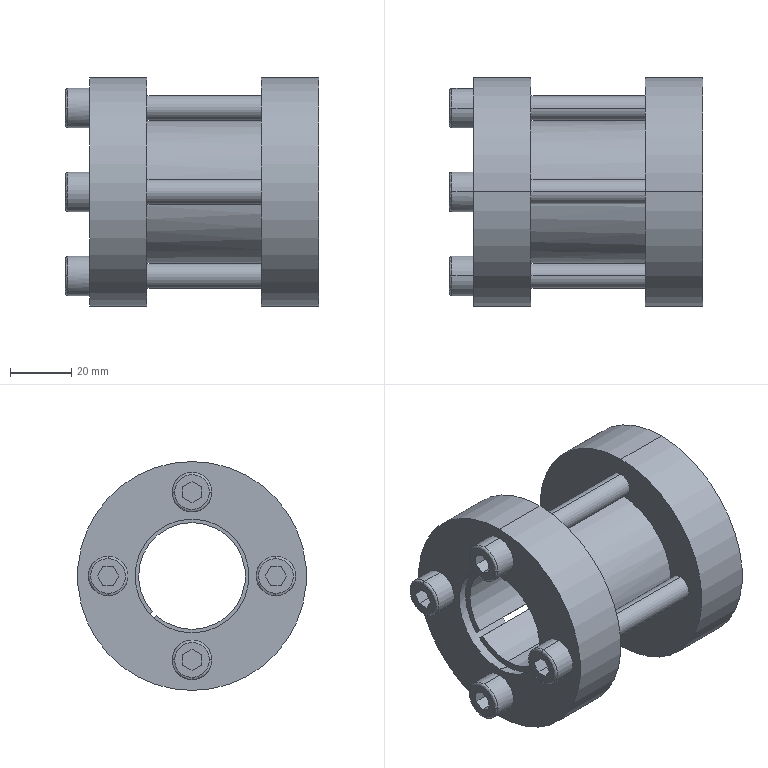Part | STEP file | IN-01-21-03 | 1 solid | 110 faces | box 83 x 75 x 75 mm | volume 165688 mm3 | plane 48 | cylinder 42 | cone 12 | spline 8 | commonest cylinder face diameters 6.466 x8 8 x8 8.4 x8 13 x8 75 x4 35 x3